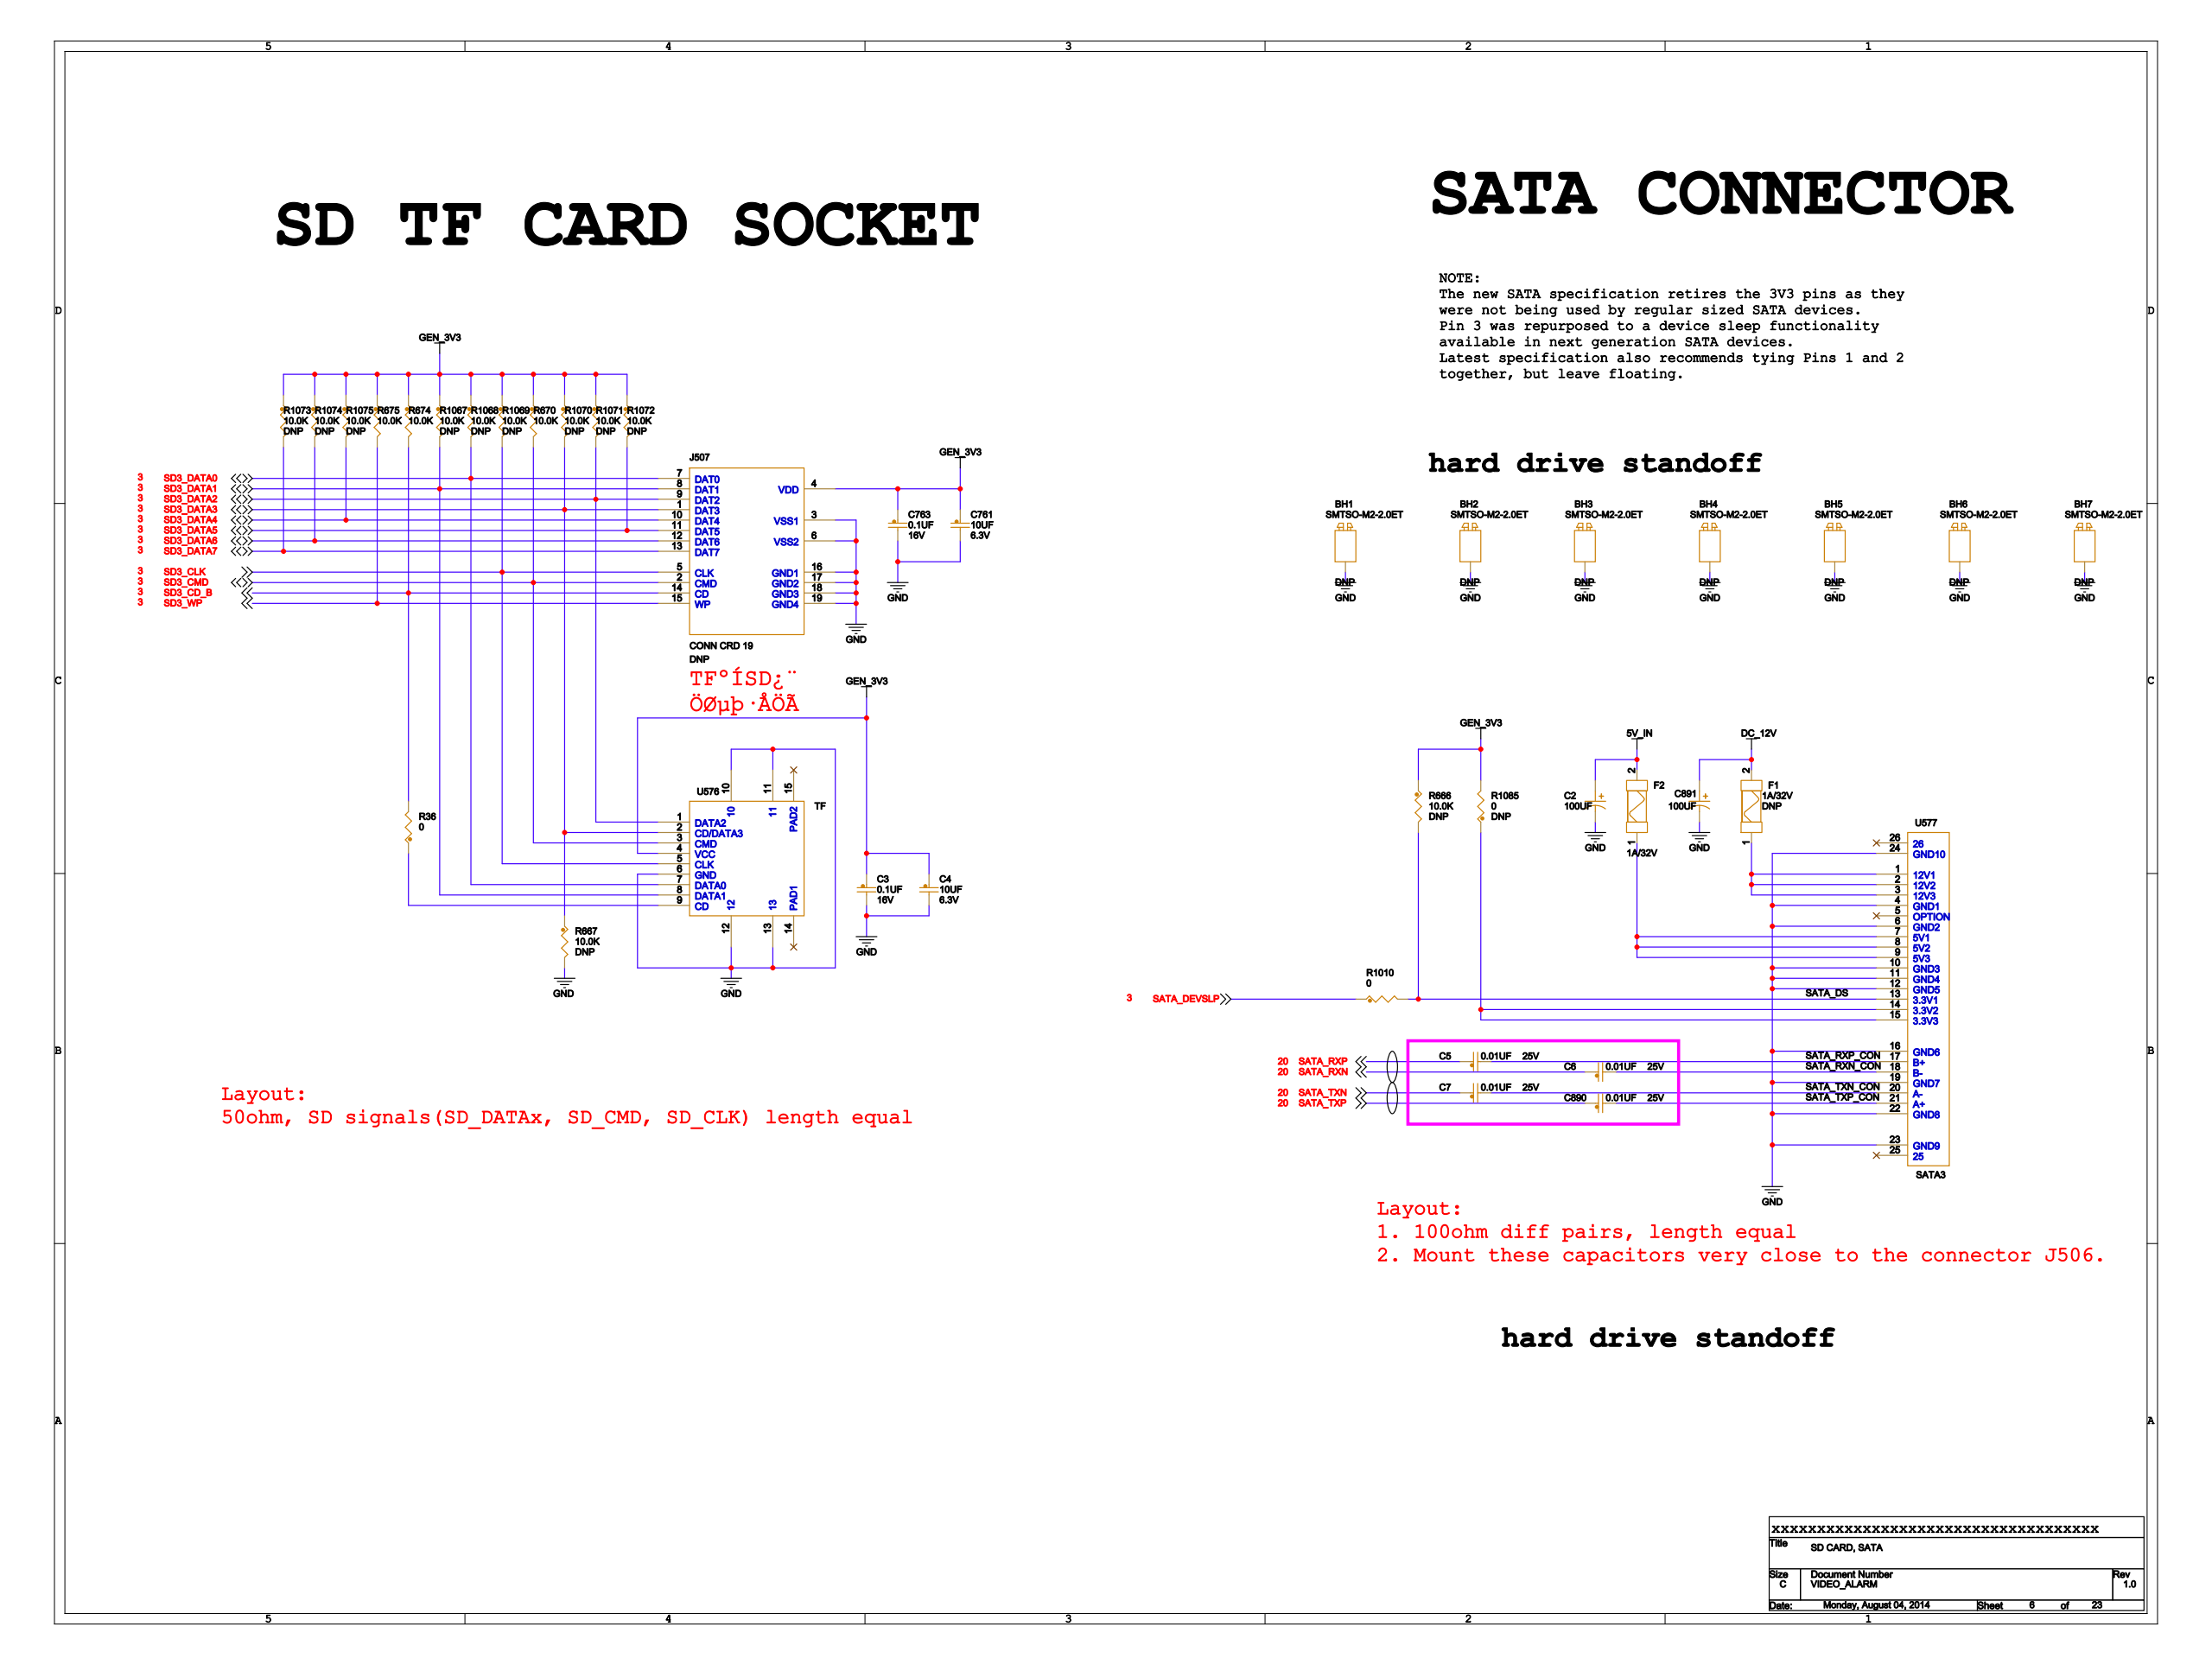Circuit board | Cadence Allegro | 994 parts | 728 nets | one sheet of the schematic
Parts on this sheet (reference | value | footprint):
BH1 | SMTSO-M2-2.0ET | HOLE_C5MM_D3MM
BH2 | SMTSO-M2-2.0ET | HOLE_C5MM_D3MM
BH3 | SMTSO-M2-2.0ET | HOLE_C5MM_D3MM
BH4 | SMTSO-M2-2.0ET | HOLE_C5MM_D3MM
BH5 | SMTSO-M2-2.0ET | HOLE_C5MM_D3MM
BH6 | SMTSO-M2-2.0ET | HOLE_C5MM_D3MM
BH7 | SMTSO-M2-2.0ET | HOLE_C5MM_D3MM
C2 | 100UF | TC6032
C4 | 10UF | 0603_CC
C5 | 0.01UF | 0603_CC
C6 | 0.01UF | 0603_CC
C7 | 0.01UF | 0603_CC
C761 | 10UF | 0603_CC
C763 | 0.1UF | 0603_CC
C890 | 0.01UF | 0603_CC
C891 | 100UF | TC7343
F1 | 1A/32V | 1206_CC
F2 | 1A/32V | 1206_CC
J507 | CONN CRD 19 | CON19_SDCARD_28X16_SM
R36 | 0 | 0603_CC
R666 | 10.0K | 0603_CC
R667 | 10.0K | 0603_CC
R670 | 10.0K | 0603_CC
R674 | 10.0K | 0603_CC
R675 | 10.0K | 0603_CC
R1010 | 0 | 0603_CC
R1067 | 10.0K | 0603_CC
R1068 | 10.0K | 0603_CC
R1069 | 10.0K | 0603_CC
R1070 | 10.0K | 0603_CC
R1071 | 10.0K | 0603_CC
R1072 | 10.0K | 0603_CC
R1073 | 10.0K | 0603_CC
R1074 | 10.0K | 0603_CC
R1075 | 10.0K | 0603_CC
R1085 | 0 | 0603_CC
U576 | TF | TF
U577 | SATA3 | SATA3
Nets of these parts (net: part-pin ...):
GND: BH1-1 BH2-1 BH3-1 BH4-1 BH5-1 BH6-1 BH7-1 C2-2 C4-2 C761-2 C763-2 C891-2 J507-3 J507-6 J507-16 J507-17 J507-18 J507-19 R667-2 U576-6 U576-10 U576-11 U576-12 U576-13 U577-4 U577-6 U577-10 U577-11 U577-12 U577-16 U577-19 U577-22 U577-23 U577-24
GEN_3V3: C4-1 C761-1 C763-1 J507-4 R666-1 R670-1 R674-1 R675-1 R1067-1 R1068-1 R1069-1 R1070-1 R1071-1 R1072-1 R1073-1 R1074-1 R1075-1 R1085-2 U576-4
DC_12V: C891-1 F1-2
5V_IN: C2-1 F2-2
N23110860: R1085-1 U577-14 U577-15
N22795504: R36-1 U576-9
SD3_CD_B: J507-14 R36-2 R674-2
SATA_DEVSLP: R1010-1
SATA_DS: R666-2 R1010-2 U577-13
SD3_WP: J507-15 R675-2
SD3_CMD: J507-2 R670-2 U576-3
SD3_DATA3: J507-1 R667-1 R1070-2 U576-2
SD3_DATA4: J507-10 R1075-2
SD3_DATA6: J507-12 R1074-2
SD3_DATA7: J507-13 R1073-2
SD3_DATA5: J507-11 R1072-2
SD3_DATA2: J507-9 R1071-2 U576-1
SD3_CLK: J507-5 R1069-2 U576-5
SD3_DATA0: J507-7 R1068-2 U576-7
SD3_DATA1: J507-8 R1067-2 U576-8
N23110566: F2-1 U577-7 U577-8 U577-9
N22505217: F1-1 U577-1 U577-2 U577-3
SATA_TXP: C890-1
SATA_TXP_CON: C890-2 U577-21
SATA_TXN: C7-1
SATA_TXN_CON: C7-2 U577-20
SATA_RXN: C6-1
SATA_RXN_CON: C6-2 U577-18
SATA_RXP: C5-1
SATA_RXP_CON: C5-2 U577-17